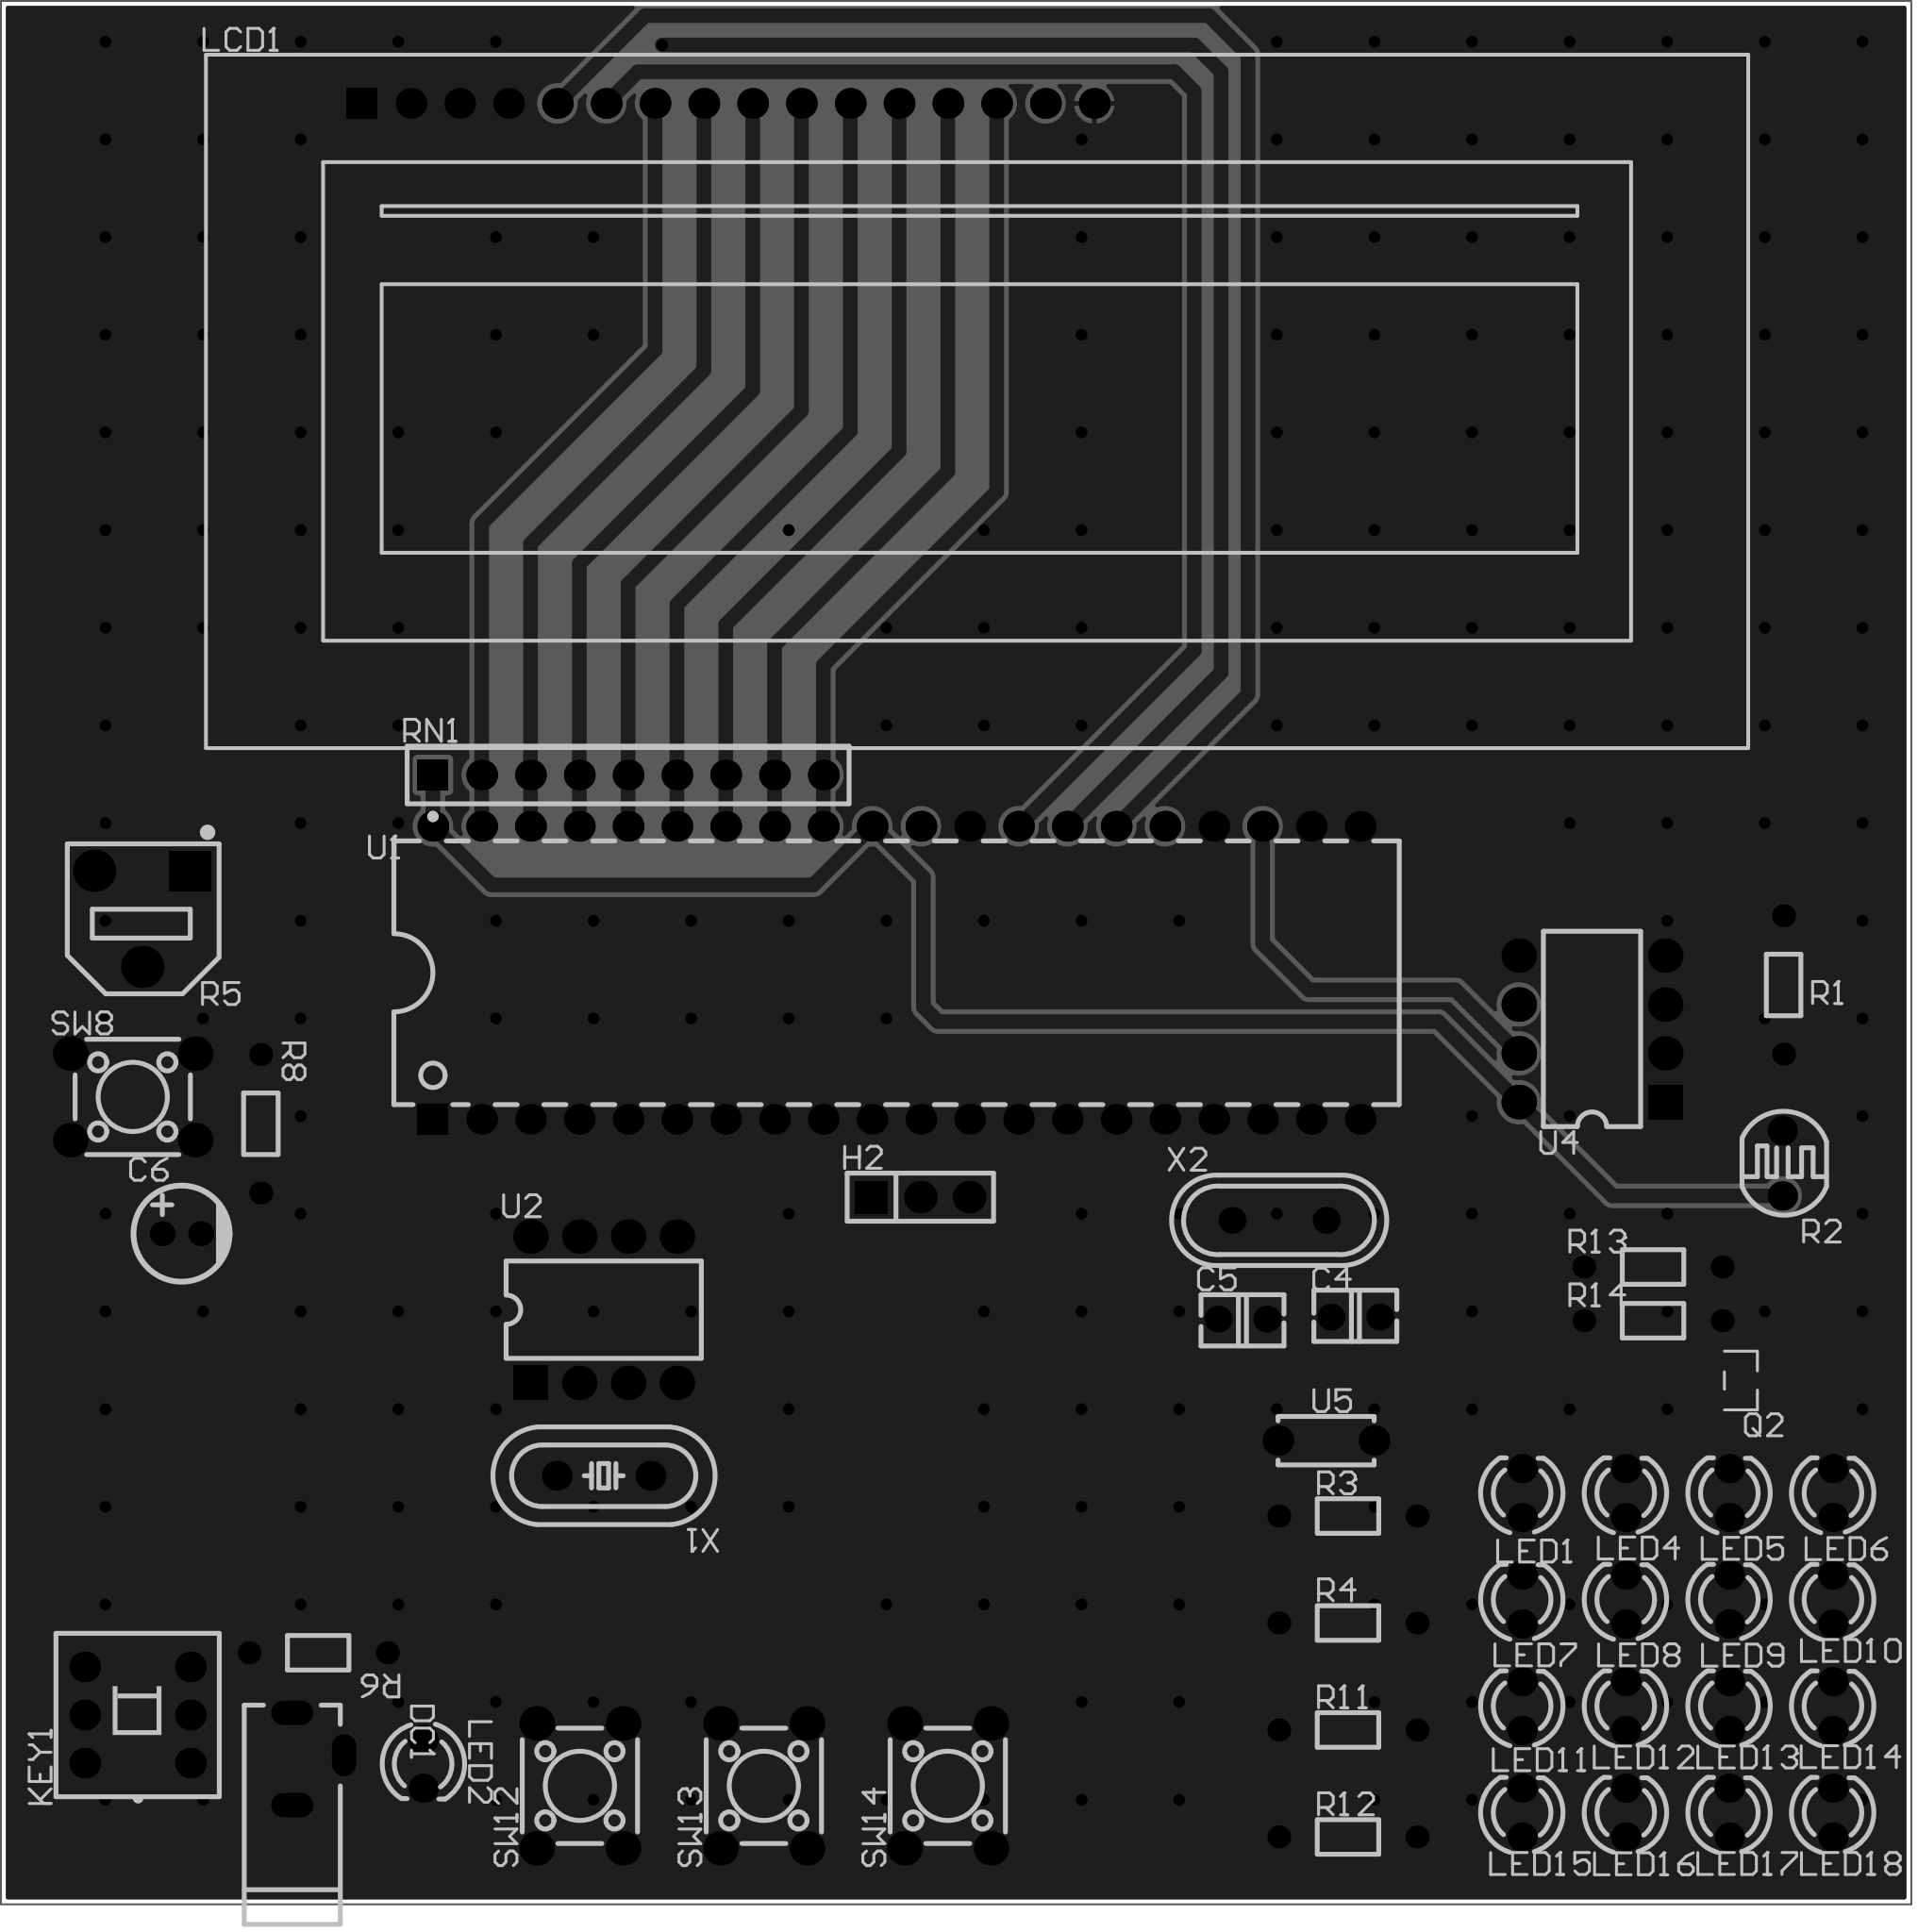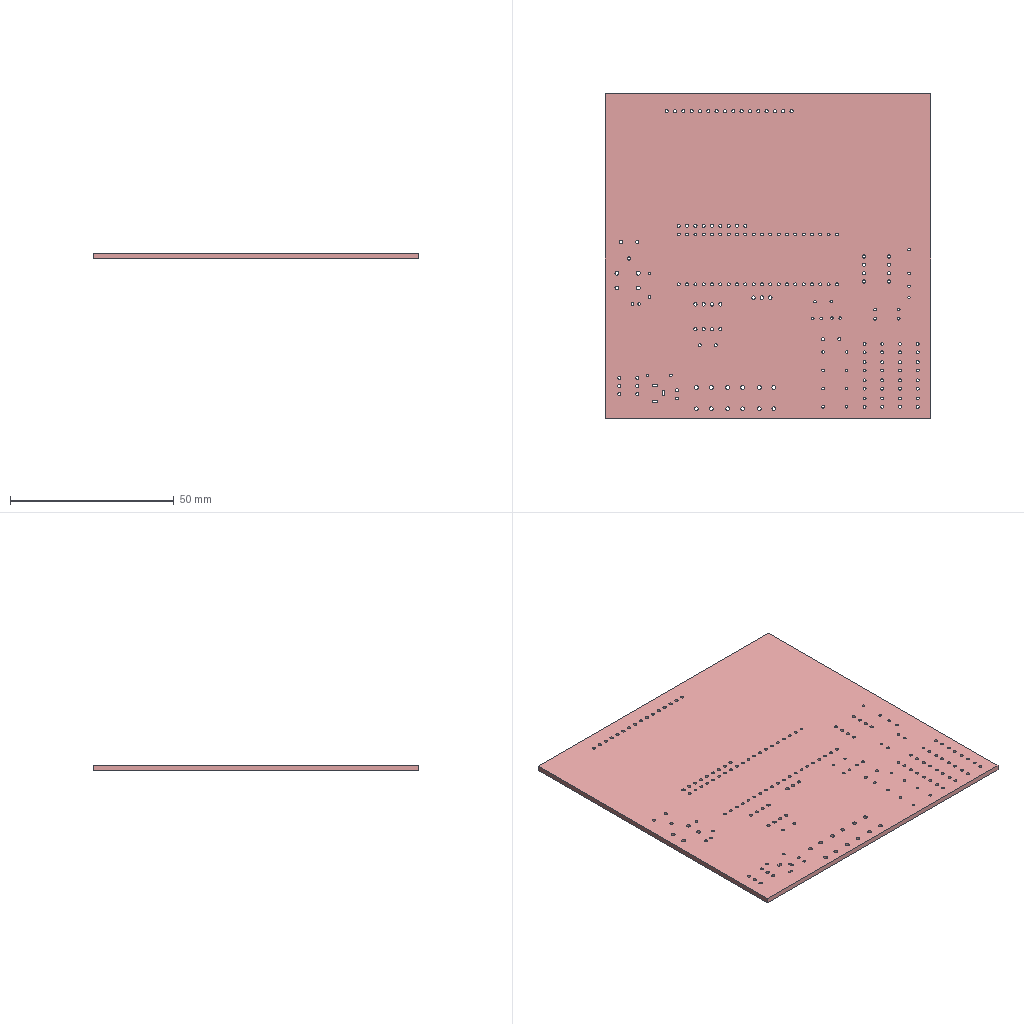Circuit board layout | Altium Designer | box 99.4 x 99 x 1.6 mm
Layer stack:
# Altium Designer layer stack of  (unit mm; dielectric type: 0 none, 1 core, 2 prepreg, 3 surface material)
index,name,kind,layer,copper_thickness_mm,dielectric_type,dielectric_thickness_mm,dielectric_material,dielectric_constant
0,Top Paste Mask Layer,other,,,,,,
1,Top Silkscreen Layer,other,,,,,,
2,Top Solder Mask Layer,dielectric,,,3,0.01,,3.3
3,Top Layer,copper,Top Layer,0.035,,,,
4,Dielectric1,dielectric,,,3,1.51,FR4,4.5
5,Bottom Layer,copper,Bottom Layer,0.035,,,,
6,Bottom Solder Mask Layer,dielectric,,,3,0.01,,3.3
7,Bottom Silkscreen Layer,other,,,,,,
8,Bottom Paste Mask Layer,other,,,,,,
# drill layer pairs: low layer,high layer
drill_pair,Top Layer,Bottom Layer
Part placement:
Designator,Comment,Layer,Footprint,Center-X(mm),Center-Y(mm),Rotation
C4,30pF,TopLayer,CAP-TH_L3.8-W2.5-P2.54-D0.50,163.195,122.301,180
C5,30pF,TopLayer,CAP-TH_L3.8-W2.5-P2.54-D0.50,157.323,122.192,0
C6,10uF,TopLayer,CAP-TH_BD5.0-P2.00-D0.8-FD-10UF50VC110GL,102.108,126.639,0
H2,,TopLayer,HDR-TH_3P-P2.54-V-M,140.559,128.536,0
KEY1,Non-latching switch 8.5×8.5 silent,TopLayer,SW-TH_6P-L8.5-W8.5-P2.54,99.822,101.6,90
LCD1,HS1602A,TopLayer,LCD1602,130.56,185.426,0
LED2,,TopLayer,LED_TH-3mm,114.681,99.06,270
R8,10kΩ,TopLayer,Res_1/8W,106.235,132.354,270
R5,10kΩ,TopLayer,RES-ADJ-SMD_RM065-V1,100.063,143.013,180
R6,1kΩ,TopLayer,Res_1/8W,109.22,104.839,180
SW8,,TopLayer,SW-TH_4P-L6.0-W6.0-P4.50-LS6.5,99.568,133.751,0
SW12,,TopLayer,SW-TH_4P-L6.0-W6.0-P4.50-LS6.5,122.839,97.917,90
SW13,,TopLayer,SW-TH_4P-L6.0-W6.0-P4.50-LS6.5,132.413,97.917,90
SW14,,TopLayer,SW-TH_4P-L6.0-W6.0-P4.50-LS6.5,141.986,97.917,90
U1,STC89C52RC-40I-PDIP40,TopLayer,DIP-40_L52.0-W13.7-P2.54-LS15.2-BL,139.319,140.208,0
X2,11.059MHz,TopLayer,OSC-TH_L11.1-W4.7-P4.88,159.228,127.331,0
DC1,DC-002,TopLayer,DC-IN-TH_DC-3510,109.22,99.314,270
LED1,,TopLayer,LED_TH-3mm,171.874,113.146,90
LED4,,TopLayer,LED_TH-3mm,177.267,113.146,90
LED5,,TopLayer,LED_TH-3mm,182.659,113.146,90
LED6,,TopLayer,LED_TH-3mm,188.051,113.146,90
LED7,,TopLayer,LED_TH-3mm,171.874,107.606,90
LED8,,TopLayer,LED_TH-3mm,177.267,107.606,90
LED9,,TopLayer,LED_TH-3mm,182.659,107.606,90
LED10,,TopLayer,LED_TH-3mm,188.051,107.606,90
LED11,,TopLayer,LED_TH-3mm,171.874,102.066,90
LED12,,TopLayer,LED_TH-3mm,177.267,102.066,90
LED13,,TopLayer,LED_TH-3mm,182.659,102.066,90
LED14,,TopLayer,LED_TH-3mm,188.051,102.066,90
LED15,,TopLayer,LED_TH-3mm,171.874,96.526,90
LED16,,TopLayer,LED_TH-3mm,177.267,96.526,90
LED17,,TopLayer,LED_TH-3mm,182.659,96.526,90
LED18,,TopLayer,LED_TH-3mm,188.051,96.526,90
Q2,BSS138,TopLayer,SOT-23-3_L3.0-W1.7-P0.95-LS2.9-BR,183.261,118.999,180
R1,10kΩ,TopLayer,Res_1/8W,185.484,139.573,90
R2,GL5549(80-100),TopLayer,RES-TH_L5.1-W4.3-P3.40-D0.5,185.42,130.302,180
R3,220Ω,TopLayer,Res_1/8W,162.814,111.95,0
R4,220Ω,TopLayer,Res_1/8W,162.814,106.386,0
R11,220Ω,TopLayer,Res_1/8W,162.814,100.822,0
R12,220Ω,TopLayer,Res_1/8W,162.814,95.258,0
R13,1kΩ,TopLayer,Res_1/8W,178.689,124.904,0
R14,10kΩ,TopLayer,Res_1/8W,178.689,122.11,0
RN1,-,TopLayer,RES-ARRAY-TH_9P-P2.54-D1.0,125.349,150.495,0
U2,DS1302N,TopLayer,DIP-8_L9.7-W6.4-P2.54-LS7.6-BL,124.079,122.682,0
U4,XPT2046,TopLayer,DIP-8_L9.7-W6.4-P2.54-LS7.6-BL,175.514,137.287,90
U5,1nF,TopLayer,CAP-TH_L5.0-W2.5-P5.00-D1.0,161.674,115.88,0
X1,32.768KHZ,TopLayer,HC-49S_L11.5-W5.0-P4.88,124.079,114.046,180
Pad and via stacks:
# Altium Designer via and pad stacks of  (unit mm). Each distinct definition once, with the count of objects using it.
# via: kind,start_layer,end_layer,hole_mm,diameter_mm,mode(0 simple;1 top-mid-bottom;2 full stack),diameter_per_layer,count,example_net
# pad: kind,layer,hole_mm,hole_type(0 round;1 square;2 slot),plating,top_size,top_shape(1 round;2 rect;3 octagon;9 rounded rect),mid_size,bottom_size,mode,footprint,size_per_layer,count,example
pad,Multi-Layer,0.8,0,plated,1.4x1.4,1,1.4x1.4,1.4x1.4,0,CAP-TH_L3.8-W2.5-P2.54-D0.50,,4,C4.1
pad,Multi-Layer,0.8,0,plated,1.3x1.3,1,1.3x1.3,1.3x1.3,0,CAP-TH_BD5.0-P2.00-D0.8-FD-10UF50VC110GL,,2,C6.2
pad,Multi-Layer,1.1,0,plated,1.7x1.7,2,1.7x1.7,1.7x1.7,0,HDR-TH_3P-P2.54-V-M,,1,H2.1
pad,Multi-Layer,1.1,0,plated,1.7x1.7,1,1.7x1.7,1.7x1.7,0,HDR-TH_3P-P2.54-V-M,,2,H2.2
pad,Multi-Layer,1,0,plated,1.6x1.6,1,1.6x1.6,1.6x1.6,0,SW-TH_6P-L8.5-W8.5-P2.54,,6,KEY1.4
pad,Multi-Layer,1,0,plated,1.6x1.6,1,1.6x1.6,1.6x1.6,0,LCD1602,,15,LCD1.16
pad,Multi-Layer,1,0,plated,1.6x1.6,2,1.6x1.6,1.6x1.6,0,LCD1602,,1,LCD1.1
pad,Multi-Layer,0.9144,0,plated,1.524x1.524,1,1.524x1.524,1.524x1.524,0,LED_TH-3mm,,34,LED2.1
pad,Multi-Layer,0.8001,0,plated,1.199x1.199,1,1.199x1.199,1.199x1.199,0,Res_1/8W,,18,R8.1
pad,Multi-Layer,1,0,plated,2.2x2.1,2,2.2x2.1,2.2x2.1,0,RES-ADJ-SMD_RM065-V1,,1,R5.1
pad,Multi-Layer,1,0,plated,2.2x2.2,1,2.2x2.2,2.2x2.2,0,RES-ADJ-SMD_RM065-V1,,2,R5.3
pad,Multi-Layer,1.2,0,plated,1.8x1.8,1,1.8x1.8,1.8x1.8,0,SW-TH_4P-L6.0-W6.0-P4.50-LS6.5,,16,SW8.1
pad,Multi-Layer,0.889,0,plated,1.6x1.6,1,1.6x1.6,1.6x1.6,0,DIP-40_L52.0-W13.7-P2.54-LS15.2-BL,,39,U1.31
pad,Multi-Layer,0.889,0,plated,1.6x1.6,2,1.6x1.6,1.6x1.6,0,DIP-40_L52.0-W13.7-P2.54-LS15.2-BL,,1,U1.1
pad,Multi-Layer,0.7,0,plated,1.4x1.4,1,1.4x1.4,1.4x1.4,0,OSC-TH_L11.1-W4.7-P4.88,,2,X2.1
pad,Multi-Layer,0.8,2,plated,2.2x1.27,1,2.2x1.27,2.2x1.27,0,DC-IN-TH_DC-3510,,3,DC1.3
pad,Multi-Layer,0.762,0,plated,1.524x1.524,1,1.524x1.524,1.524x1.524,0,RES-TH_L5.1-W4.3-P3.40-D0.5,,2,R2.2
pad,Multi-Layer,1,0,plated,1.6x1.6,2,1.6x1.6,1.6x1.6,0,RES-ARRAY-TH_9P-P2.54-D1.0,,1,RN1.1
pad,Multi-Layer,1,0,plated,1.6x1.6,1,1.6x1.6,1.6x1.6,0,RES-ARRAY-TH_9P-P2.54-D1.0,,8,RN1.2
pad,Multi-Layer,1,0,plated,1.8x1.8,2,1.8x1.8,1.8x1.8,0,DIP-8_L9.7-W6.4-P2.54-LS7.6-BL,,2,U2.1
pad,Multi-Layer,1,0,plated,1.8x1.8,1,1.8x1.8,1.8x1.8,0,DIP-8_L9.7-W6.4-P2.54-LS7.6-BL,,14,U2.2
pad,Multi-Layer,1,0,plated,1.6x1.6,1,1.6x1.6,1.6x1.6,0,CAP-TH_L5.0-W2.5-P5.00-D1.0,,2,U5.1
pad,Multi-Layer,0.9,0,plated,1.56x1.56,1,1.56x1.56,1.56x1.56,0,HC-49S_L11.5-W5.0-P4.88,,2,X1.1
pad,Top Layer,0,0,plated,1.038x0.532,2,1.038x0.532,1.038x0.532,0,SOT-23-3_L3.0-W1.7-P0.95-LS2.9-BR,,3,Q2.1
via,Top Layer,Bottom Layer,0.3048,0.61,0,,226,P26
Copper pours:
name,layer,net,type(0 solid;1 hatched;2 none)
Top Layer-GND,Top Layer,GND,0
Bottom Layer-GND,Bottom Layer,GND,0
Design rules, without the lines most boards share:
# Altium Designer design rules of  (exported by Altium Designer, unit mm)
# columns: name | kind | enabled | priority | scope1 | scope2 | descriptor | typed fields (field=value)
creepage | 65 | enabled | 1 | All | All | Creepage Distance Constraint =(0mil) (All),(All) |
copperRegion | 20 | enabled | 1 | (InNet('GND')) | All | Polygon Connect Rule(Relief Connect )(Conductor Width=10mil) (Relief Angle=90 Angle) (Entries=4) (Air Gap Width=10mil) ((InNet('GND'))),(All) | connect_style(0=relief,1=direct,2=none)=0 relief_conductor_width=0.254 relief_entries=4